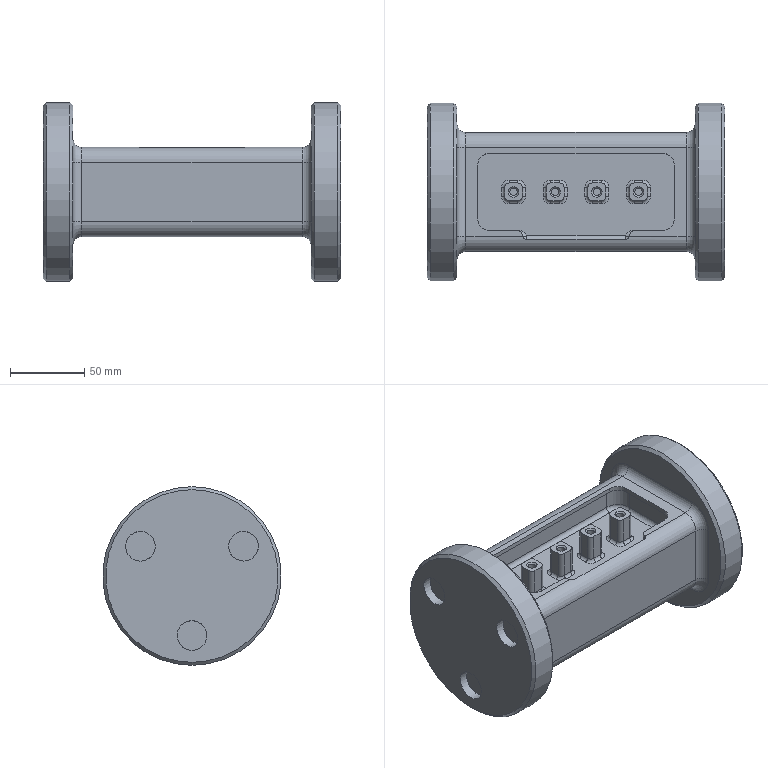CAM job | NX | 3-axis milling | part box 200 x 120 x 120 mm | stock box 200 x 120 x 120 mm
Tools:
number,name,description,diameter,corner_radius,flute_length,length,flutes
1,D12R1,Milling Tool-5 Parameters,12.0,1.0,50.0,75.0,2
0,CXD,Milling Tool-T Cutter,15.0,,6.0,25.0,4
0,PD,Milling Tool-5 Parameters,30.0,0.8,50.0,75.0,2
0,D10,Milling Tool-5 Parameters,10.0,0.0,50.0,75.0,2
0,D10R1,Milling Tool-5 Parameters,10.0,1.0,50.0,75.0,2
0,PERSON_A_T_TOOL,Milling Tool-T Cutter,16.0,,6.0,40.0,4
Operations:
program,operation,operation_type,tool,method,geometry_group,spindle_rpm,surface_speed,feed_per_tooth,feed_cut,feed_plunge,cut_length_mm,path_length_mm,cut_time_min,machine_time_min
NC_PROGRAM,PLANAR_MILL,PlanarMilling,PD,METHOD,WORKPIECE,4000.0,376.0,0.125,1000.0,100.0,532.0,606.0,0.532,0.5394
NC_PROGRAM,CAVITY_MILL,CavityMilling,D12R1,METHOD,WORKPIECE,0.0,0.0,0.0,250.0,100.0,12047.572,12422.571,48.19,48.228
NC_PROGRAM,PLANAR_MILL_1,PlanarMilling,D10,METHOD,WORKPIECE,0.0,0.0,0.0,250.0,100.0,1254.017,1373.417,5.016,5.028
NC_PROGRAM,ZLEVEL_PROFILE,ZLevelMilling,D10R1,METHOD,WORKPIECE,0.0,0.0,0.0,250.0,100.0,11742.336,12212.389,46.969,47.016
NC_PROGRAM,ZLEVEL_PROFILE_COPY,ZLevelMilling,CXD,METHOD,WORKPIECE,0.0,0.0,0.0,250.0,100.0,3681.63,3785.13,14.726,14.737
NC_PROGRAM,CONTOUR_SURFACE_AREA,SurfaceContour,PERSON_A_T_TOOL,METHOD,MCS_MILL,3000.0,282.0,0.4167,2500.0,100.0,8563.999,8593.999,3.426,3.429
NC_PROGRAM,CONTOUR_SURFACE_AREA_COPY,SurfaceContour,PERSON_A_T_TOOL,METHOD,MCS_MILL,3000.0,282.0,0.4167,2500.0,100.0,3380.528,3410.928,1.352,1.355
NC_PROGRAM,CONTOUR_SURFACE_AREA_COPY_1,SurfaceContour,PERSON_A_T_TOOL,METHOD,MCS_MILL,3000.0,282.0,0.4167,2500.0,100.0,1693.773,1705.773,0.6775,0.6787
NC_PROGRAM,CONTOUR_SURFACE_AREA_COPY_1_COPY,SurfaceContour,PERSON_A_T_TOOL,METHOD,MCS_MILL,3000.0,282.0,0.4167,2500.0,100.0,8486.769,8516.769,3.395,3.398